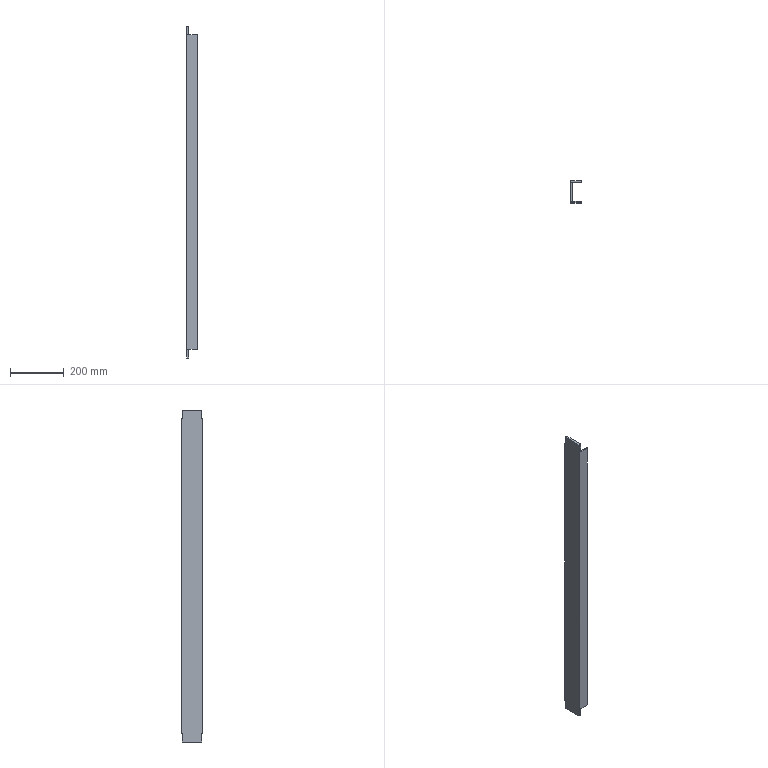Part | SolidWorks | features Cut 3, LPattern 2, Extrusion 1, SheetMetal 1 | 1 solid | 68 faces | box 40 x 80 x 1232 mm | volume 1071667 mm3 | plane 38 | cylinder 30 | commonest cylinder face diameters 9 x30